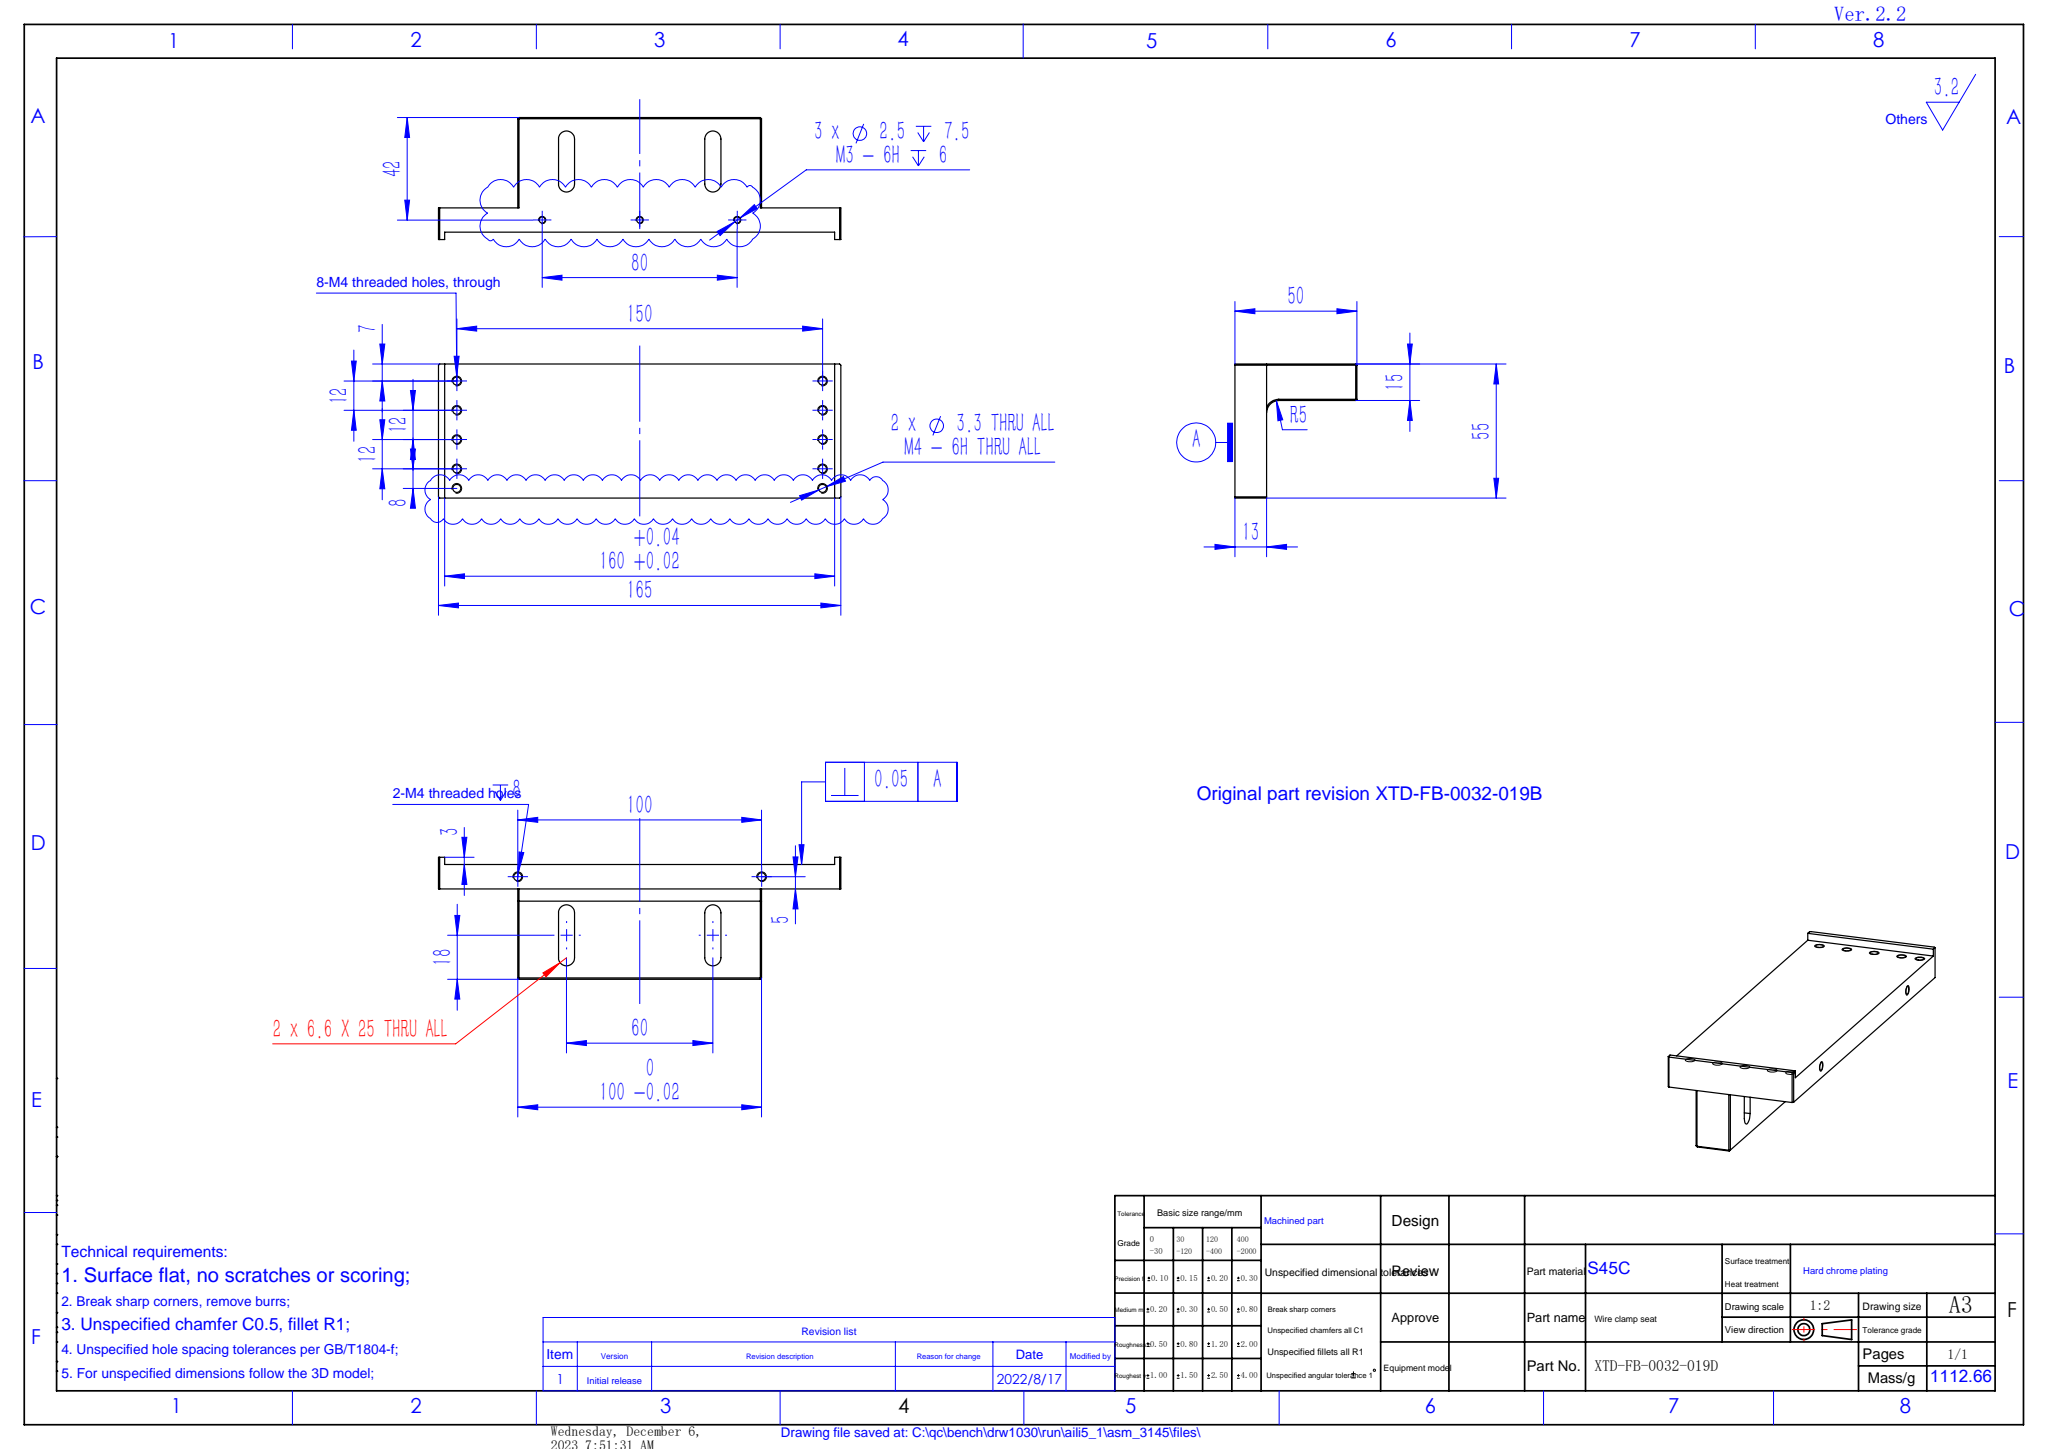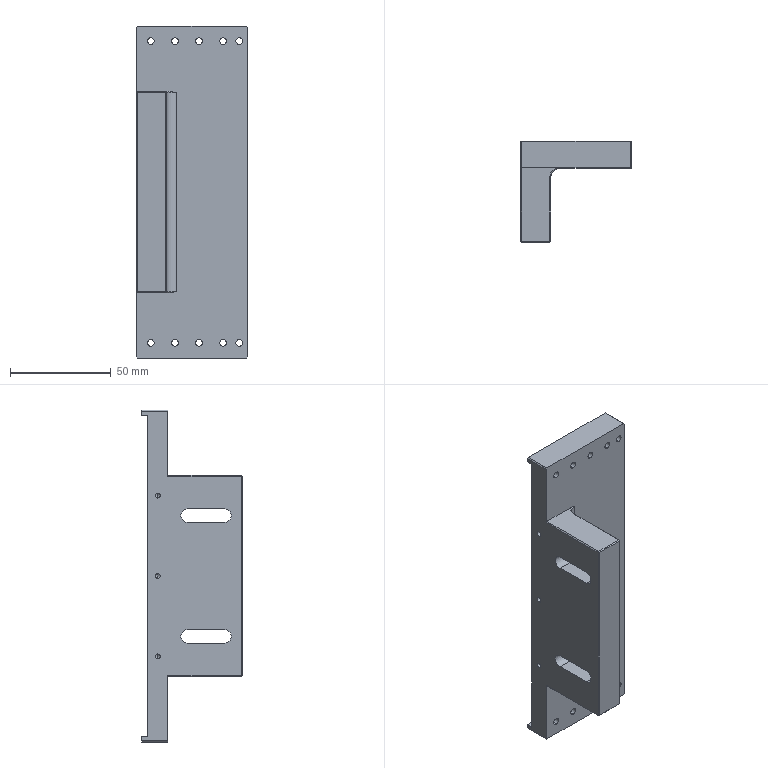Part | SolidWorks | features HoleWzd 5, ICE 2, Chamfer 1, Extrusion 1 | 1 solid | 81 faces | box 55 x 50 x 165 mm | volume 141740 mm3 | cylinder 35 | plane 34 | cone 12 | commonest cylinder face diameters 3.3 x24 2.5 x6 6.6 x4 10 x1